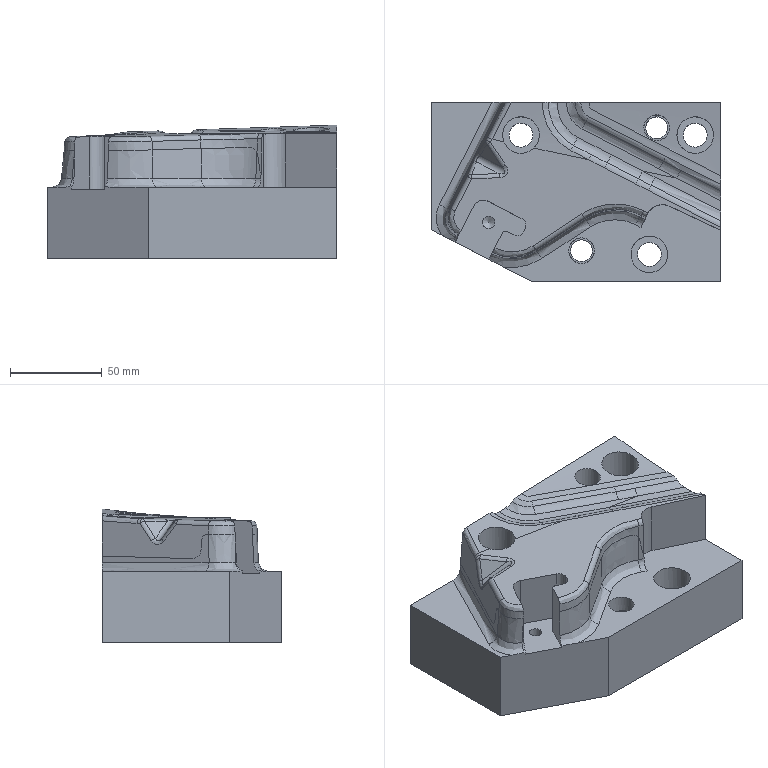Part | STEP file | gslz 2016.10.28-13_id1630_x_t | 1 solid | 103 faces | box 158 x 98 x 72.916 mm | volume 768512 mm3 | spline 51 | cylinder 27 | plane 22 | sphere 2 | cone 1 | commonest cylinder face diameters 5.5 x10 12 x3 13 x3 20 x3 8 x2 14 x2